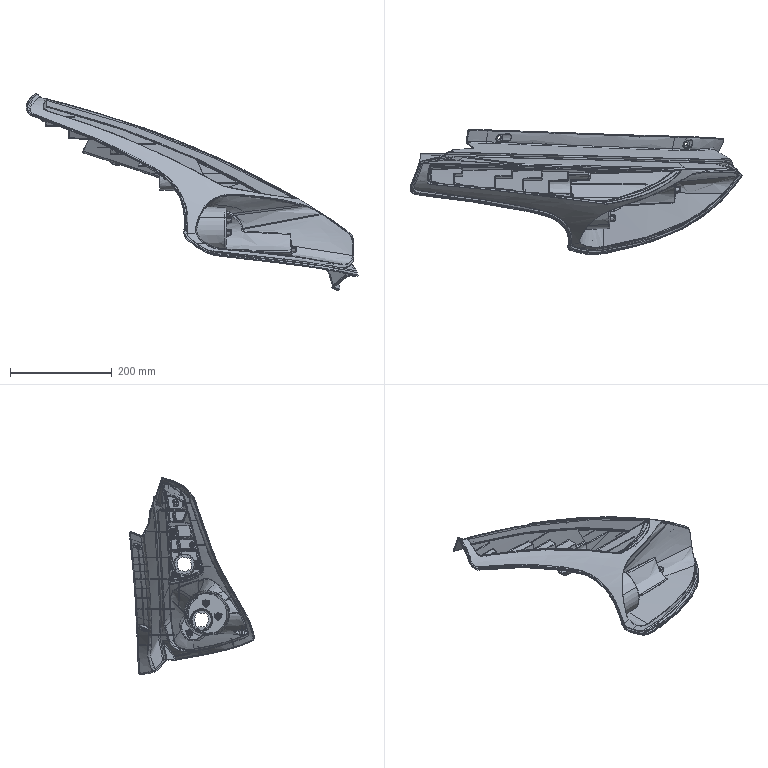Part | STEP file | solid 194 | 1 solid | 1858 faces | box 652.487 x 245.902 x 387.851 mm | volume 656196 mm3 | spline 1392 | plane 215 | sphere 85 | cylinder 72 | torus 44 | cone 41 | other 9 | commonest cylinder face diameters 2.01 x17 4.02 x17 27.135 x8 31.155 x8 2.915 x7 1.005 x6